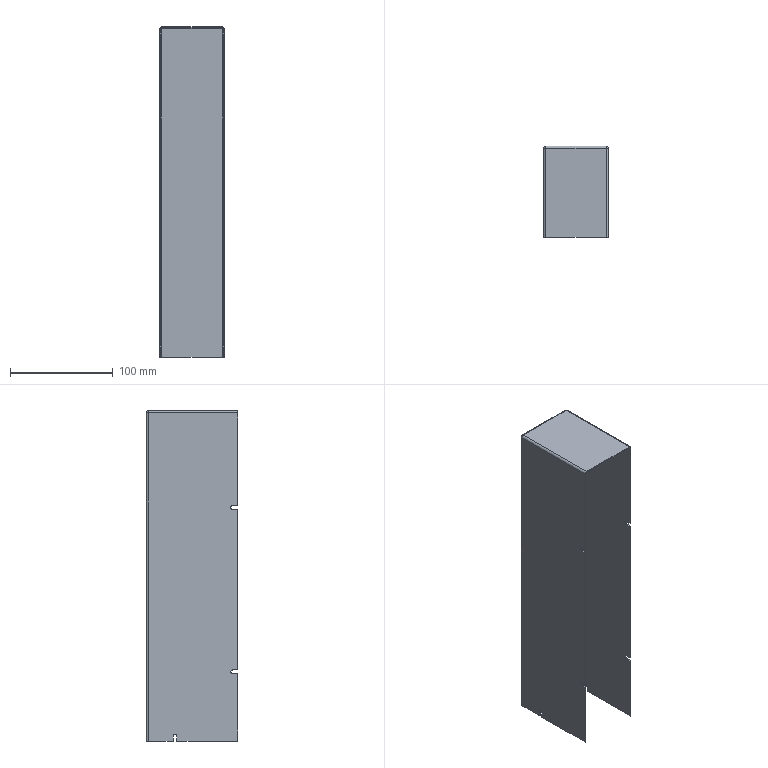Part | NX | features BREP 1 | 1 solid | 48 faces | box 63 x 89 x 321.5 mm | volume 81505 mm3 | plane 28 | cylinder 16 | sphere 4 | commonest cylinder face diameters 3.5 x6 2 x5 4 x5
STEP:
#1=CARTESIAN_POINT('',(30.5,14.75,0.));
#2=VERTEX_POINT('',#1);
#3=CARTESIAN_POINT('',(30.5,14.75,5.));
#4=VERTEX_POINT('',#3);
#5=CARTESIAN_POINT('',(30.5,14.75,321.5));
#6=DIRECTION('',(0.,0.,1.));
#7=VECTOR('',#6,1000.);
#8=LINE('',#5,#7);
#9=EDGE_CURVE('',#2,#4,#8,.T.);
#10=ORIENTED_EDGE('',*,*,#9,.T.);
#11=CARTESIAN_POINT('',(31.5,14.75,5.));
#12=VERTEX_POINT('',#11);
#13=CARTESIAN_POINT('',(-31.5,14.75,5.));
#14=DIRECTION('',(1.,0.,0.));
#15=VECTOR('',#14,1000.);
#16=LINE('',#13,#15);
#17=EDGE_CURVE('',#4,#12,#16,.T.);
#18=ORIENTED_EDGE('',*,*,#17,.T.);
#19=CARTESIAN_POINT('',(31.5,14.75,0.));
#20=VERTEX_POINT('',#19);
#21=CARTESIAN_POINT('',(31.5,14.75,5.));
#22=DIRECTION('',(0.,0.,-1.));
#23=VECTOR('',#22,1000.);
#24=LINE('',#21,#23);
#25=EDGE_CURVE('',#12,#20,#24,.T.);
#26=ORIENTED_EDGE('',*,*,#25,.T.);
#27=CARTESIAN_POINT('',(-31.5,14.75,0.));
#28=DIRECTION('',(1.,0.,0.));
#29=VECTOR('',#28,1000.);
#30=LINE('',#27,#29);
#31=EDGE_CURVE('',#2,#20,#30,.T.);
#32=ORIENTED_EDGE('',*,*,#31,.F.);
#33=EDGE_LOOP('',(#10,#18,#26,#32));
#34=FACE_BOUND('',#33,.T.);
#35=CARTESIAN_POINT('',(-31.5,14.75,5.));
#36=DIRECTION('',(0.,-1.,0.));
#37=DIRECTION('',(0.,0.,-1.));
#38=AXIS2_PLACEMENT_3D('',#35,#36,#37);
#39=PLANE('',#38);
#40=ADVANCED_FACE('',(#34),#39,.F.);
#41=CARTESIAN_POINT('',(30.5,18.25,5.));
#42=VERTEX_POINT('',#41);
#43=CARTESIAN_POINT('',(30.5,18.25,0.));
#44=VERTEX_POINT('',#43);
#45=CARTESIAN_POINT('',(30.5,18.25,321.5));
#46=DIRECTION('',(0.,0.,-1.));
#47=VECTOR('',#46,1000.);
#48=LINE('',#45,#47);
#49=EDGE_CURVE('',#42,#44,#48,.T.);
#50=ORIENTED_EDGE('',*,*,#49,.T.);
#51=CARTESIAN_POINT('',(31.5,18.25,0.));
#52=VERTEX_POINT('',#51);
#53=CARTESIAN_POINT('',(-31.5,18.25,0.));
#54=DIRECTION('',(1.,0.,0.));
#55=VECTOR('',#54,1000.);
#56=LINE('',#53,#55);
#57=EDGE_CURVE('',#44,#52,#56,.T.);
#58=ORIENTED_EDGE('',*,*,#57,.T.);
#59=CARTESIAN_POINT('',(31.5,18.25,5.));
#60=VERTEX_POINT('',#59);
#61=CARTESIAN_POINT('',(31.5,18.25,5.));
#62=DIRECTION('',(0.,0.,1.));
#63=VECTOR('',#62,1000.);
#64=LINE('',#61,#63);
#65=EDGE_CURVE('',#52,#60,#64,.T.);
#66=ORIENTED_EDGE('',*,*,#65,.T.);
#67=CARTESIAN_POINT('',(-31.5,18.25,5.));
#68=DIRECTION('',(1.,0.,0.));
#69=VECTOR('',#68,1000.);
#70=LINE('',#67,#69);
#71=EDGE_CURVE('',#42,#60,#70,.T.);
#72=ORIENTED_EDGE('',*,*,#71,.F.);
#73=EDGE_LOOP('',(#50,#58,#66,#72));
#74=FACE_BOUND('',#73,.T.);
#75=CARTESIAN_POINT('',(-31.5,18.25,5.));
#76=DIRECTION('',(0.,1.,0.));
#77=DIRECTION('',(0.,0.,1.));
#78=AXIS2_PLACEMENT_3D('',#75,#76,#77);
#79=PLANE('',#78);
#80=ADVANCED_FACE('',(#74),#79,.F.);
#81=CARTESIAN_POINT('',(30.5,16.5,5.));
#82=DIRECTION('',(-1.,0.,0.));
#83=DIRECTION('',(0.,0.,1.));
#84=AXIS2_PLACEMENT_3D('',#81,#82,#83);
#85=CIRCLE('',#84,1.75);
#86=EDGE_CURVE('',#4,#42,#85,.T.);
#87=ORIENTED_EDGE('',*,*,#86,.T.);
#88=ORIENTED_EDGE('',*,*,#71,.T.);
#89=CARTESIAN_POINT('',(31.5,16.5,5.));
#90=DIRECTION('',(1.,0.,0.));
#91=DIRECTION('',(0.,0.,-1.));
#92=AXIS2_PLACEMENT_3D('',#89,#90,#91);
#93=CIRCLE('',#92,1.75);
#94=EDGE_CURVE('',#60,#12,#93,.T.);
#95=ORIENTED_EDGE('',*,*,#94,.T.);
#96=ORIENTED_EDGE('',*,*,#17,.F.);
#97=EDGE_LOOP('',(#87,#88,#95,#96));
#98=FACE_BOUND('',#97,.T.);
#99=CARTESIAN_POINT('',(-31.5,16.5,5.));
#100=DIRECTION('',(1.,0.,0.));
#101=DIRECTION('',(0.,0.,-1.));
#102=AXIS2_PLACEMENT_3D('',#99,#100,#101);
#103=CYLINDRICAL_SURFACE('',#102,1.75);
#104=ADVANCED_FACE('',(#98),#103,.F.);
#105=CARTESIAN_POINT('',(30.5,-44.5,69.25));
#106=VERTEX_POINT('',#105);
#107=CARTESIAN_POINT('',(30.5,-39.5,69.25));
#108=VERTEX_POINT('',#107);
#109=CARTESIAN_POINT('',(30.5,-44.5,69.25));
#110=DIRECTION('',(0.,1.,0.));
#111=VECTOR('',#110,1000.);
#112=LINE('',#109,#111);
#113=EDGE_CURVE('',#106,#108,#112,.T.);
#114=ORIENTED_EDGE('',*,*,#113,.T.);
#115=CARTESIAN_POINT('',(31.5,-39.5,69.25));
#116=VERTEX_POINT('',#115);
#117=CARTESIAN_POINT('',(-31.5,-39.5,69.25));
#118=DIRECTION('',(1.,0.,0.));
#119=VECTOR('',#118,1000.);
#120=LINE('',#117,#119);
#121=EDGE_CURVE('',#108,#116,#120,.T.);
#122=ORIENTED_EDGE('',*,*,#121,.T.);
#123=CARTESIAN_POINT('',(31.5,-44.5,69.25));
#124=VERTEX_POINT('',#123);
#125=CARTESIAN_POINT('',(31.5,-39.5,69.25));
#126=DIRECTION('',(0.,-1.,0.));
#127=VECTOR('',#126,1000.);
#128=LINE('',#125,#127);
#129=EDGE_CURVE('',#116,#124,#128,.T.);
#130=ORIENTED_EDGE('',*,*,#129,.T.);
#131=CARTESIAN_POINT('',(-31.5,-44.5,69.25));
#132=DIRECTION('',(1.,0.,0.));
#133=VECTOR('',#132,1000.);
#134=LINE('',#131,#133);
#135=EDGE_CURVE('',#106,#124,#134,.T.);
#136=ORIENTED_EDGE('',*,*,#135,.F.);
#137=EDGE_LOOP('',(#114,#122,#130,#136));
#138=FACE_BOUND('',#137,.T.);
#139=CARTESIAN_POINT('',(-31.5,-39.5,69.25));
#140=DIRECTION('',(0.,0.,1.));
#141=DIRECTION('',(0.,-1.,0.));
#142=AXIS2_PLACEMENT_3D('',#139,#140,#141);
#143=PLANE('',#142);
#144=ADVANCED_FACE('',(#138),#143,.F.);
#145=CARTESIAN_POINT('',(30.5,-39.5,65.75));
#146=VERTEX_POINT('',#145);
#147=CARTESIAN_POINT('',(30.5,-44.5,65.75));
#148=VERTEX_POINT('',#147);
#149=CARTESIAN_POINT('',(30.5,-44.5,65.75));
#150=DIRECTION('',(0.,-1.,0.));
#151=VECTOR('',#150,1000.);
#152=LINE('',#149,#151);
#153=EDGE_CURVE('',#146,#148,#152,.T.);
#154=ORIENTED_EDGE('',*,*,#153,.T.);
#155=CARTESIAN_POINT('',(31.5,-44.5,65.75));
#156=VERTEX_POINT('',#155);
#157=CARTESIAN_POINT('',(-31.5,-44.5,65.75));
#158=DIRECTION('',(1.,0.,0.));
#159=VECTOR('',#158,1000.);
#160=LINE('',#157,#159);
#161=EDGE_CURVE('',#148,#156,#160,.T.);
#162=ORIENTED_EDGE('',*,*,#161,.T.);
#163=CARTESIAN_POINT('',(31.5,-39.5,65.75));
#164=VERTEX_POINT('',#163);
#165=CARTESIAN_POINT('',(31.5,-39.5,65.75));
#166=DIRECTION('',(0.,1.,0.));
#167=VECTOR('',#166,1000.);
#168=LINE('',#165,#167);
#169=EDGE_CURVE('',#156,#164,#168,.T.);
#170=ORIENTED_EDGE('',*,*,#169,.T.);
#171=CARTESIAN_POINT('',(-31.5,-39.5,65.75));
#172=DIRECTION('',(1.,0.,0.));
#173=VECTOR('',#172,1000.);
#174=LINE('',#171,#173);
#175=EDGE_CURVE('',#146,#164,#174,.T.);
#176=ORIENTED_EDGE('',*,*,#175,.F.);
#177=EDGE_LOOP('',(#154,#162,#170,#176));
#178=FACE_BOUND('',#177,.T.);
#179=CARTESIAN_POINT('',(-31.5,-39.5,65.75));
#180=DIRECTION('',(0.,0.,-1.));
#181=DIRECTION('',(0.,1.,0.));
#182=AXIS2_PLACEMENT_3D('',#179,#180,#181);
#183=PLANE('',#182);
#184=ADVANCED_FACE('',(#178),#183,.F.);
#185=CARTESIAN_POINT('',(30.5,-39.5,67.5));
#186=DIRECTION('',(-1.,0.,0.));
#187=DIRECTION('',(0.,0.,1.));
#188=AXIS2_PLACEMENT_3D('',#185,#186,#187);
#189=CIRCLE('',#188,1.75);
#190=EDGE_CURVE('',#108,#146,#189,.T.);
#191=ORIENTED_EDGE('',*,*,#190,.T.);
#192=ORIENTED_EDGE('',*,*,#175,.T.);
#193=CARTESIAN_POINT('',(31.5,-39.5,67.5));
#194=DIRECTION('',(1.,0.,0.));
#195=DIRECTION('',(0.,0.,-1.));
#196=AXIS2_PLACEMENT_3D('',#193,#194,#195);
#197=CIRCLE('',#196,1.75);
#198=EDGE_CURVE('',#164,#116,#197,.T.);
#199=ORIENTED_EDGE('',*,*,#198,.T.);
#200=ORIENTED_EDGE('',*,*,#121,.F.);
#201=EDGE_LOOP('',(#191,#192,#199,#200));
#202=FACE_BOUND('',#201,.T.);
#203=CARTESIAN_POINT('',(-31.5,-39.5,67.5));
#204=DIRECTION('',(1.,0.,0.));
#205=DIRECTION('',(0.,0.,-1.));
#206=AXIS2_PLACEMENT_3D('',#203,#204,#205);
#207=CYLINDRICAL_SURFACE('',#206,1.75);
#208=ADVANCED_FACE('',(#202),#207,.F.);
#209=CARTESIAN_POINT('',(-30.5,18.25,5.));
#210=VERTEX_POINT('',#209);
#211=CARTESIAN_POINT('',(-30.5,14.75,5.));
#212=VERTEX_POINT('',#211);
#213=CARTESIAN_POINT('',(-30.5,16.5,5.));
#214=DIRECTION('',(1.,0.,0.));
#215=DIRECTION('',(0.,0.,-1.));
#216=AXIS2_PLACEMENT_3D('',#213,#214,#215);
#217=CIRCLE('',#216,1.75);
#218=EDGE_CURVE('',#210,#212,#217,.T.);
#219=ORIENTED_EDGE('',*,*,#218,.T.);
#220=CARTESIAN_POINT('',(-31.5,14.75,5.));
#221=VERTEX_POINT('',#220);
#222=CARTESIAN_POINT('',(-31.5,14.75,5.));
#223=DIRECTION('',(1.,0.,0.));
#224=VECTOR('',#223,1000.);
#225=LINE('',#222,#224);
#226=EDGE_CURVE('',#221,#212,#225,.T.);
#227=ORIENTED_EDGE('',*,*,#226,.F.);
#228=CARTESIAN_POINT('',(-31.5,18.25,5.));
#229=VERTEX_POINT('',#228);
#230=CARTESIAN_POINT('',(-31.5,16.5,5.));
#231=DIRECTION('',(1.,0.,0.));
#232=DIRECTION('',(0.,0.,-1.));
#233=AXIS2_PLACEMENT_3D('',#230,#231,#232);
#234=CIRCLE('',#233,1.75);
#235=EDGE_CURVE('',#229,#221,#234,.T.);
#236=ORIENTED_EDGE('',*,*,#235,.F.);
#237=CARTESIAN_POINT('',(-31.5,18.25,5.));
#238=DIRECTION('',(1.,0.,0.));
#239=VECTOR('',#238,1000.);
#240=LINE('',#237,#239);
#241=EDGE_CURVE('',#229,#210,#240,.T.);
#242=ORIENTED_EDGE('',*,*,#241,.T.);
#243=EDGE_LOOP('',(#219,#227,#236,#242));
#244=FACE_BOUND('',#243,.T.);
#245=CARTESIAN_POINT('',(-31.5,16.5,5.));
#246=DIRECTION('',(1.,0.,0.));
#247=DIRECTION('',(0.,0.,-1.));
#248=AXIS2_PLACEMENT_3D('',#245,#246,#247);
#249=CYLINDRICAL_SURFACE('',#248,1.75);
#250=ADVANCED_FACE('',(#244),#249,.F.);
#251=CARTESIAN_POINT('',(-30.5,18.25,0.));
#252=VERTEX_POINT('',#251);
#253=CARTESIAN_POINT('',(-30.5,18.25,321.5));
#254=DIRECTION('',(0.,0.,1.));
#255=VECTOR('',#254,1000.);
#256=LINE('',#253,#255);
#257=EDGE_CURVE('',#252,#210,#256,.T.);
#258=ORIENTED_EDGE('',*,*,#257,.T.);
#259=ORIENTED_EDGE('',*,*,#241,.F.);
#260=CARTESIAN_POINT('',(-31.5,18.25,0.));
#261=VERTEX_POINT('',#260);
#262=CARTESIAN_POINT('',(-31.5,18.25,5.));
#263=DIRECTION('',(0.,0.,1.));
#264=VECTOR('',#263,1000.);
#265=LINE('',#262,#264);
#266=EDGE_CURVE('',#261,#229,#265,.T.);
#267=ORIENTED_EDGE('',*,*,#266,.F.);
#268=CARTESIAN_POINT('',(-31.5,18.25,0.));
#269=DIRECTION('',(1.,0.,0.));
#270=VECTOR('',#269,1000.);
#271=LINE('',#268,#270);
#272=EDGE_CURVE('',#261,#252,#271,.T.);
#273=ORIENTED_EDGE('',*,*,#272,.T.);
#274=EDGE_LOOP('',(#258,#259,#267,#273));
#275=FACE_BOUND('',#274,.T.);
#276=CARTESIAN_POINT('',(-31.5,18.25,5.));
#277=DIRECTION('',(0.,1.,0.));
#278=DIRECTION('',(0.,0.,1.));
#279=AXIS2_PLACEMENT_3D('',#276,#277,#278);
#280=PLANE('',#279);
#281=ADVANCED_FACE('',(#275),#280,.F.);
#282=CARTESIAN_POINT('',(-30.5,14.75,0.));
#283=VERTEX_POINT('',#282);
#284=CARTESIAN_POINT('',(-30.5,14.75,321.5));
#285=DIRECTION('',(0.,0.,-1.));
#286=VECTOR('',#285,1000.);
#287=LINE('',#284,#286);
#288=EDGE_CURVE('',#212,#283,#287,.T.);
#289=ORIENTED_EDGE('',*,*,#288,.T.);
#290=CARTESIAN_POINT('',(-31.5,14.75,0.));
#291=VERTEX_POINT('',#290);
#292=CARTESIAN_POINT('',(-31.5,14.75,0.));
#293=DIRECTION('',(1.,0.,0.));
#294=VECTOR('',#293,1000.);
#295=LINE('',#292,#294);
#296=EDGE_CURVE('',#291,#283,#295,.T.);
#297=ORIENTED_EDGE('',*,*,#296,.F.);
#298=CARTESIAN_POINT('',(-31.5,14.75,5.));
#299=DIRECTION('',(0.,0.,-1.));
#300=VECTOR('',#299,1000.);
#301=LINE('',#298,#300);
#302=EDGE_CURVE('',#221,#291,#301,.T.);
#303=ORIENTED_EDGE('',*,*,#302,.F.);
#304=ORIENTED_EDGE('',*,*,#226,.T.);
#305=EDGE_LOOP('',(#289,#297,#303,#304));
#306=FACE_BOUND('',#305,.T.);
#307=CARTESIAN_POINT('',(-31.5,14.75,5.));
#308=DIRECTION('',(0.,-1.,0.));
#309=DIRECTION('',(0.,0.,-1.));
#310=AXIS2_PLACEMENT_3D('',#307,#308,#309);
#311=PLANE('',#310);
#312=ADVANCED_FACE('',(#306),#311,.F.);
#313=CARTESIAN_POINT('',(-30.5,-39.5,65.75));
#314=VERTEX_POINT('',#313);
#315=CARTESIAN_POINT('',(-30.5,-39.5,69.25));
#316=VERTEX_POINT('',#315);
#317=CARTESIAN_POINT('',(-30.5,-39.5,67.5));
#318=DIRECTION('',(1.,0.,0.));
#319=DIRECTION('',(0.,0.,-1.));
#320=AXIS2_PLACEMENT_3D('',#317,#318,#319);
#321=CIRCLE('',#320,1.75);
#322=EDGE_CURVE('',#314,#316,#321,.T.);
#323=ORIENTED_EDGE('',*,*,#322,.T.);
#324=CARTESIAN_POINT('',(-31.5,-39.5,69.25));
#325=VERTEX_POINT('',#324);
#326=CARTESIAN_POINT('',(-31.5,-39.5,69.25));
#327=DIRECTION('',(1.,0.,0.));
#328=VECTOR('',#327,1000.);
#329=LINE('',#326,#328);
#330=EDGE_CURVE('',#325,#316,#329,.T.);
#331=ORIENTED_EDGE('',*,*,#330,.F.);
#332=CARTESIAN_POINT('',(-31.5,-39.5,65.75));
#333=VERTEX_POINT('',#332);
#334=CARTESIAN_POINT('',(-31.5,-39.5,67.5));
#335=DIRECTION('',(1.,0.,0.));
#336=DIRECTION('',(0.,0.,-1.));
#337=AXIS2_PLACEMENT_3D('',#334,#335,#336);
#338=CIRCLE('',#337,1.75);
#339=EDGE_CURVE('',#333,#325,#338,.T.);
#340=ORIENTED_EDGE('',*,*,#339,.F.);
#341=CARTESIAN_POINT('',(-31.5,-39.5,65.75));
#342=DIRECTION('',(1.,0.,0.));
#343=VECTOR('',#342,1000.);
#344=LINE('',#341,#343);
#345=EDGE_CURVE('',#333,#314,#344,.T.);
#346=ORIENTED_EDGE('',*,*,#345,.T.);
#347=EDGE_LOOP('',(#323,#331,#340,#346));
#348=FACE_BOUND('',#347,.T.);
#349=CARTESIAN_POINT('',(-31.5,-39.5,67.5));
#350=DIRECTION('',(1.,0.,0.));
#351=DIRECTION('',(0.,0.,-1.));
#352=AXIS2_PLACEMENT_3D('',#349,#350,#351);
#353=CYLINDRICAL_SURFACE('',#352,1.75);
#354=ADVANCED_FACE('',(#348),#353,.F.);
#355=CARTESIAN_POINT('',(-30.5,-44.5,65.75));
#356=VERTEX_POINT('',#355);
#357=CARTESIAN_POINT('',(-30.5,-44.5,65.75));
#358=DIRECTION('',(0.,1.,0.));
#359=VECTOR('',#358,1000.);
#360=LINE('',#357,#359);
#361=EDGE_CURVE('',#356,#314,#360,.T.);
#362=ORIENTED_EDGE('',*,*,#361,.T.);
#363=ORIENTED_EDGE('',*,*,#345,.F.);
#364=CARTESIAN_POINT('',(-31.5,-44.5,65.75));
#365=VERTEX_POINT('',#364);
#366=CARTESIAN_POINT('',(-31.5,-39.5,65.75));
#367=DIRECTION('',(0.,1.,0.));
#368=VECTOR('',#367,1000.);
#369=LINE('',#366,#368);
#370=EDGE_CURVE('',#365,#333,#369,.T.);
#371=ORIENTED_EDGE('',*,*,#370,.F.);
#372=CARTESIAN_POINT('',(-31.5,-44.5,65.75));
#373=DIRECTION('',(1.,0.,0.));
#374=VECTOR('',#373,1000.);
#375=LINE('',#372,#374);
#376=EDGE_CURVE('',#365,#356,#375,.T.);
#377=ORIENTED_EDGE('',*,*,#376,.T.);
#378=EDGE_LOOP('',(#362,#363,#371,#377));
#379=FACE_BOUND('',#378,.T.);
#380=CARTESIAN_POINT('',(-31.5,-39.5,65.75));
#381=DIRECTION('',(0.,0.,-1.));
#382=DIRECTION('',(0.,1.,0.));
#383=AXIS2_PLACEMENT_3D('',#380,#381,#382);
#384=PLANE('',#383);
#385=ADVANCED_FACE('',(#379),#384,.F.);
#386=CARTESIAN_POINT('',(-30.5,-44.5,69.25));
#387=VERTEX_POINT('',#386);
#388=CARTESIAN_POINT('',(-30.5,-44.5,69.25));
#389=DIRECTION('',(0.,-1.,0.));
#390=VECTOR('',#389,1000.);
#391=LINE('',#388,#390);
#392=EDGE_CURVE('',#316,#387,#391,.T.);
#393=ORIENTED_EDGE('',*,*,#392,.T.);
#394=CARTESIAN_POINT('',(-31.5,-44.5,69.25));
#395=VERTEX_POINT('',#394);
#396=CARTESIAN_POINT('',(-31.5,-44.5,69.25));
#397=DIRECTION('',(1.,0.,0.));
#398=VECTOR('',#397,1000.);
#399=LINE('',#396,#398);
#400=EDGE_CURVE('',#395,#387,#399,.T.);
#401=ORIENTED_EDGE('',*,*,#400,.F.);
#402=CARTESIAN_POINT('',(-31.5,-39.5,69.25));
#403=DIRECTION('',(0.,-1.,0.));
#404=VECTOR('',#403,1000.);
#405=LINE('',#402,#404);
#406=EDGE_CURVE('',#325,#395,#405,.T.);
#407=ORIENTED_EDGE('',*,*,#406,.F.);
#408=ORIENTED_EDGE('',*,*,#330,.T.);
#409=EDGE_LOOP('',(#393,#401,#407,#408));
#410=FACE_BOUND('',#409,.T.);
#411=CARTESIAN_POINT('',(-31.5,-39.5,69.25));
#412=DIRECTION('',(0.,0.,1.));
#413=DIRECTION('',(0.,-1.,0.));
#414=AXIS2_PLACEMENT_3D('',#411,#412,#413);
#415=PLANE('',#414);
#416=ADVANCED_FACE('',(#410),#415,.F.);
#417=CARTESIAN_POINT('',(30.5,-39.5,225.75));
#418=VERTEX_POINT('',#417);
#419=CARTESIAN_POINT('',(30.5,-44.5,225.75));
#420=VERTEX_POINT('',#419);
#421=CARTESIAN_POINT('',(30.5,-44.5,225.75));
#422=DIRECTION('',(0.,-1.,0.));
#423=VECTOR('',#422,1000.);
#424=LINE('',#421,#423);
#425=EDGE_CURVE('',#418,#420,#424,.T.);
#426=ORIENTED_EDGE('',*,*,#425,.T.);
#427=CARTESIAN_POINT('',(31.5,-44.5,225.75));
#428=VERTEX_POINT('',#427);
#429=CARTESIAN_POINT('',(-31.5,-44.5,225.75));
#430=DIRECTION('',(1.,0.,0.));
#431=VECTOR('',#430,1000.);
#432=LINE('',#429,#431);
#433=EDGE_CURVE('',#420,#428,#432,.T.);
#434=ORIENTED_EDGE('',*,*,#433,.T.);
#435=CARTESIAN_POINT('',(31.5,-39.5,225.75));
#436=VERTEX_POINT('',#435);
#437=CARTESIAN_POINT('',(31.5,-44.5,225.75));
#438=DIRECTION('',(0.,1.,0.));
#439=VECTOR('',#438,1000.);
#440=LINE('',#437,#439);
#441=EDGE_CURVE('',#428,#436,#440,.T.);
#442=ORIENTED_EDGE('',*,*,#441,.T.);
#443=CARTESIAN_POINT('',(-31.5,-39.5,225.75));
#444=DIRECTION('',(1.,0.,0.));
#445=VECTOR('',#444,1000.);
#446=LINE('',#443,#445);
#447=EDGE_CURVE('',#418,#436,#446,.T.);
#448=ORIENTED_EDGE('',*,*,#447,.F.);
#449=EDGE_LOOP('',(#426,#434,#442,#448));
#450=FACE_BOUND('',#449,.T.);
#451=CARTESIAN_POINT('',(-31.5,-44.5,225.75));
#452=DIRECTION('',(0.,0.,-1.));
#453=DIRECTION('',(0.,1.,0.));
#454=AXIS2_PLACEMENT_3D('',#451,#452,#453);
#455=PLANE('',#454);
#456=ADVANCED_FACE('',(#450),#455,.F.);
#457=CARTESIAN_POINT('',(30.5,-39.5,229.25));
#458=VERTEX_POINT('',#457);
#459=CARTESIAN_POINT('',(30.5,-39.5,227.5));
#460=DIRECTION('',(-1.,0.,0.));
#461=DIRECTION('',(0.,0.,1.));
#462=AXIS2_PLACEMENT_3D('',#459,#460,#461);
#463=CIRCLE('',#462,1.75);
#464=EDGE_CURVE('',#458,#418,#463,.T.);
#465=ORIENTED_EDGE('',*,*,#464,.T.);
#466=ORIENTED_EDGE('',*,*,#447,.T.);
#467=CARTESIAN_POINT('',(31.5,-39.5,229.25));
#468=VERTEX_POINT('',#467);
#469=CARTESIAN_POINT('',(31.5,-39.5,227.5));
#470=DIRECTION('',(1.,0.,0.));
#471=DIRECTION('',(0.,0.,-1.));
#472=AXIS2_PLACEMENT_3D('',#469,#470,#471);
#473=CIRCLE('',#472,1.75);
#474=EDGE_CURVE('',#436,#468,#473,.T.);
#475=ORIENTED_EDGE('',*,*,#474,.T.);
#476=CARTESIAN_POINT('',(-31.5,-39.5,229.25));
#477=DIRECTION('',(1.,0.,0.));
#478=VECTOR('',#477,1000.);
#479=LINE('',#476,#478);
#480=EDGE_CURVE('',#458,#468,#479,.T.);
#481=ORIENTED_EDGE('',*,*,#480,.F.);
#482=EDGE_LOOP('',(#465,#466,#475,#481));
#483=FACE_BOUND('',#482,.T.);
#484=CARTESIAN_POINT('',(-31.5,-39.5,227.5));
#485=DIRECTION('',(1.,0.,0.));
#486=DIRECTION('',(0.,0.,-1.));
#487=AXIS2_PLACEMENT_3D('',#484,#485,#486);
#488=CYLINDRICAL_SURFACE('',#487,1.75);
#489=ADVANCED_FACE('',(#483),#488,.F.);
#490=CARTESIAN_POINT('',(30.5,-44.5,229.25));
#491=VERTEX_POINT('',#490);
#492=CARTESIAN_POINT('',(30.5,-44.5,229.25));
#493=DIRECTION('',(0.,1.,0.));
#494=VECTOR('',#493,1000.);
#495=LINE('',#492,#494);
#496=EDGE_CURVE('',#491,#458,#495,.T.);
#497=ORIENTED_EDGE('',*,*,#496,.T.);
#498=ORIENTED_EDGE('',*,*,#480,.T.);
#499=CARTESIAN_POINT('',(31.5,-44.5,229.25));
#500=VERTEX_POINT('',#499);
#501=CARTESIAN_POINT('',(31.5,-44.5,229.25));
#502=DIRECTION('',(0.,-1.,0.));
#503=VECTOR('',#502,1000.);
#504=LINE('',#501,#503);
#505=EDGE_CURVE('',#468,#500,#504,.T.);
#506=ORIENTED_EDGE('',*,*,#505,.T.);
#507=CARTESIAN_POINT('',(-31.5,-44.5,229.25));
#508=DIRECTION('',(1.,0.,0.));
#509=VECTOR('',#508,1000.);
#510=LINE('',#507,#509);
#511=EDGE_CURVE('',#491,#500,#510,.T.);
#512=ORIENTED_EDGE('',*,*,#511,.F.);
#513=EDGE_LOOP('',(#497,#498,#506,#512));
#514=FACE_BOUND('',#513,.T.);
#515=CARTESIAN_POINT('',(-31.5,-44.5,229.25));
#516=DIRECTION('',(0.,0.,1.));
#517=DIRECTION('',(0.,-1.,0.));
#518=AXIS2_PLACEMENT_3D('',#515,#516,#517);
#519=PLANE('',#518);
#520=ADVANCED_FACE('',(#514),#519,.F.);
#521=CARTESIAN_POINT('',(-30.5,-39.5,229.25));
#522=VERTEX_POINT('',#521);
#523=CARTESIAN_POINT('',(-30.5,-44.5,229.25));
#524=VERTEX_POINT('',#523);
#525=CARTESIAN_POINT('',(-30.5,-44.5,229.25));
#526=DIRECTION('',(0.,-1.,0.));
#527=VECTOR('',#526,1000.);
#528=LINE('',#525,#527);
#529=EDGE_CURVE('',#522,#524,#528,.T.);
#530=ORIENTED_EDGE('',*,*,#529,.T.);
#531=CARTESIAN_POINT('',(-31.5,-44.5,229.25));
#532=VERTEX_POINT('',#531);
#533=CARTESIAN_POINT('',(-31.5,-44.5,229.25));
#534=DIRECTION('',(1.,0.,0.));
#535=VECTOR('',#534,1000.);
#536=LINE('',#533,#535);
#537=EDGE_CURVE('',#532,#524,#536,.T.);
#538=ORIENTED_EDGE('',*,*,#537,.F.);
#539=CARTESIAN_POINT('',(-31.5,-39.5,229.25));
#540=VERTEX_POINT('',#539);
#541=CARTESIAN_POINT('',(-31.5,-44.5,229.25));
#542=DIRECTION('',(0.,-1.,0.));
#543=VECTOR('',#542,1000.);
#544=LINE('',#541,#543);
#545=EDGE_CURVE('',#540,#532,#544,.T.);
#546=ORIENTED_EDGE('',*,*,#545,.F.);
#547=CARTESIAN_POINT('',(-31.5,-39.5,229.25));
#548=DIRECTION('',(1.,0.,0.));
#549=VECTOR('',#548,1000.);
#550=LINE('',#547,#549);
#551=EDGE_CURVE('',#540,#522,#550,.T.);
#552=ORIENTED_EDGE('',*,*,#551,.T.);
#553=EDGE_LOOP('',(#530,#538,#546,#552));
#554=FACE_BOUND('',#553,.T.);
#555=CARTESIAN_POINT('',(-31.5,-44.5,229.25));
#556=DIRECTION('',(0.,0.,1.));
#557=DIRECTION('',(0.,-1.,0.));
#558=AXIS2_PLACEMENT_3D('',#555,#556,#557);
#559=PLANE('',#558);
#560=ADVANCED_FACE('',(#554),#559,.F.);
#561=CARTESIAN_POINT('',(-30.5,-39.5,225.75));
#562=VERTEX_POINT('',#561);
#563=CARTESIAN_POINT('',(-30.5,-39.5,227.5));
#564=DIRECTION('',(1.,0.,0.));
#565=DIRECTION('',(0.,0.,-1.));
#566=AXIS2_PLACEMENT_3D('',#563,#564,#565);
#567=CIRCLE('',#566,1.75);
#568=EDGE_CURVE('',#562,#522,#567,.T.);
#569=ORIENTED_EDGE('',*,*,#568,.T.);
#570=ORIENTED_EDGE('',*,*,#551,.F.);
#571=CARTESIAN_POINT('',(-31.5,-39.5,225.75));
#572=VERTEX_POINT('',#571);
#573=CARTESIAN_POINT('',(-31.5,-39.5,227.5));
#574=DIRECTION('',(1.,0.,0.));
#575=DIRECTION('',(0.,0.,-1.));
#576=AXIS2_PLACEMENT_3D('',#573,#574,#575);
#577=CIRCLE('',#576,1.75);
#578=EDGE_CURVE('',#572,#540,#577,.T.);
#579=ORIENTED_EDGE('',*,*,#578,.F.);
#580=CARTESIAN_POINT('',(-31.5,-39.5,225.75));
#581=DIRECTION('',(1.,0.,0.));
#582=VECTOR('',#581,1000.);
#583=LINE('',#580,#582);
#584=EDGE_CURVE('',#572,#562,#583,.T.);
#585=ORIENTED_EDGE('',*,*,#584,.T.);
#586=EDGE_LOOP('',(#569,#570,#579,#585));
#587=FACE_BOUND('',#586,.T.);
#588=CARTESIAN_POINT('',(-31.5,-39.5,227.5));
#589=DIRECTION('',(1.,0.,0.));
#590=DIRECTION('',(0.,0.,-1.));
#591=AXIS2_PLACEMENT_3D('',#588,#589,#590);
#592=CYLINDRICAL_SURFACE('',#591,1.75);
#593=ADVANCED_FACE('',(#587),#592,.F.);
#594=CARTESIAN_POINT('',(-30.5,-44.5,225.75));
#595=VERTEX_POINT('',#594);
#596=CARTESIAN_POINT('',(-30.5,-44.5,225.75));
#597=DIRECTION('',(0.,1.,0.));
#598=VECTOR('',#597,1000.);
#599=LINE('',#596,#598);
#600=EDGE_CURVE('',#595,#562,#599,.T.);
#601=ORIENTED_EDGE('',*,*,#600,.T.);
#602=ORIENTED_EDGE('',*,*,#584,.F.);
#603=CARTESIAN_POINT('',(-31.5,-44.5,225.75));
#604=VERTEX_POINT('',#603);
#605=CARTESIAN_POINT('',(-31.5,-44.5,225.75));
#606=DIRECTION('',(0.,1.,0.));
#607=VECTOR('',#606,1000.);
#608=LINE('',#605,#607);
#609=EDGE_CURVE('',#604,#572,#608,.T.);
#610=ORIENTED_EDGE('',*,*,#609,.F.);
#611=CARTESIAN_POINT('',(-31.5,-44.5,225.75));
#612=DIRECTION('',(1.,0.,0.));
#613=VECTOR('',#612,1000.);
#614=LINE('',#611,#613);
#615=EDGE_CURVE('',#604,#595,#614,.T.);
#616=ORIENTED_EDGE('',*,*,#615,.T.);
#617=EDGE_LOOP('',(#601,#602,#610,#616));
#618=FACE_BOUND('',#617,.T.);
#619=CARTESIAN_POINT('',(-31.5,-44.5,225.75));
#620=DIRECTION('',(0.,0.,-1.));
#621=DIRECTION('',(0.,1.,0.));
#622=AXIS2_PLACEMENT_3D('',#619,#620,#621);
#623=PLANE('',#622);
#624=ADVANCED_FACE('',(#618),#623,.F.);
#625=CARTESIAN_POINT('',(29.5,42.5,320.5));
#626=VERTEX_POINT('',#625);
#627=CARTESIAN_POINT('',(29.5,43.5,319.5));
#628=VERTEX_POINT('',#627);
#629=CARTESIAN_POINT('',(29.5,42.5,319.5));
#630=DIRECTION('',(-1.,0.,0.));
#631=DIRECTION('',(0.,0.,1.));
#632=AXIS2_PLACEMENT_3D('',#629,#630,#631);
#633=CIRCLE('',#632,1.);
#634=EDGE_CURVE('',#626,#628,#633,.T.);
#635=ORIENTED_EDGE('',*,*,#634,.F.);
#636=CARTESIAN_POINT('',(-29.5,42.5,320.5));
#637=VERTEX_POINT('',#636);
#638=CARTESIAN_POINT('',(0.,42.5,320.5));
#639=DIRECTION('',(-1.,0.,0.));
#640=VECTOR('',#639,1000.);
#641=LINE('',#638,#640);
#642=EDGE_CURVE('',#626,#637,#641,.T.);
#643=ORIENTED_EDGE('',*,*,#642,.T.);
#644=CARTESIAN_POINT('',(-29.5,43.5,319.5));
#645=VERTEX_POINT('',#644);
#646=CARTESIAN_POINT('',(-29.5,42.5,319.5));
#647=DIRECTION('',(1.,0.,0.));
#648=DIRECTION('',(0.,0.,1.));
#649=AXIS2_PLACEMENT_3D('',#646,#647,#648);
#650=CIRCLE('',#649,1.);
#651=EDGE_CURVE('',#645,#637,#650,.T.);
#652=ORIENTED_EDGE('',*,*,#651,.F.);
#653=CARTESIAN_POINT('',(-31.5,43.5,319.5));
#654=DIRECTION('',(1.,0.,0.));
#655=VECTOR('',#654,1000.);
#656=LINE('',#653,#655);
#657=EDGE_CURVE('',#645,#628,#656,.T.);
#658=ORIENTED_EDGE('',*,*,#657,.T.);
#659=EDGE_LOOP('',(#635,#643,#652,#658));
#660=FACE_BOUND('',#659,.T.);
#661=CARTESIAN_POINT('',(0.,42.5,319.5));
#662=DIRECTION('',(-1.,0.,0.));
#663=DIRECTION('',(0.,0.,1.));
#664=AXIS2_PLACEMENT_3D('',#661,#662,#663);
#665=CYLINDRICAL_SURFACE('',#664,1.);
#666=ADVANCED_FACE('',(#660),#665,.F.);
#667=CARTESIAN_POINT('',(-30.5,42.5,319.5));
#668=VERTEX_POINT('',#667);
#669=CARTESIAN_POINT('',(-29.5,42.5,319.5));
#670=DIRECTION('',(0.,0.,1.));
#671=DIRECTION('',(1.,0.,0.));
#672=AXIS2_PLACEMENT_3D('',#669,#670,#671);
#673=CIRCLE('',#672,1.);
#674=EDGE_CURVE('',#645,#668,#673,.T.);
#675=ORIENTED_EDGE('',*,*,#674,.F.);
#676=ORIENTED_EDGE('',*,*,#651,.T.);
#677=CARTESIAN_POINT('',(-29.5,42.5,319.5));
#678=DIRECTION('',(0.,1.,0.));
#679=DIRECTION('',(-1.,0.,0.));
#680=AXIS2_PLACEMENT_3D('',#677,#678,#679);
#681=CIRCLE('',#680,1.);
#682=EDGE_CURVE('',#668,#637,#681,.T.);
#683=ORIENTED_EDGE('',*,*,#682,.F.);
#684=EDGE_LOOP('',(#675,#676,#683));
#685=FACE_BOUND('',#684,.T.);
#686=CARTESIAN_POINT('',(-29.5,42.5,319.5));
#687=DIRECTION('',(0.,1.,0.));
#688=DIRECTION('',(1.,0.,0.));
#689=AXIS2_PLACEMENT_3D('',#686,#687,#688);
#690=SPHERICAL_SURFACE('',#689,1.);
#691=ADVANCED_FACE('',(#685),#690,.F.);
#692=CARTESIAN_POINT('',(30.5,42.5,319.5));
#693=VERTEX_POINT('',#692);
#694=CARTESIAN_POINT('',(29.5,42.5,319.5));
#695=DIRECTION('',(0.,1.,0.));
#696=DIRECTION('',(0.,0.,-1.));
#697=AXIS2_PLACEMENT_3D('',#694,#695,#696);
#698=CIRCLE('',#697,1.);
#699=EDGE_CURVE('',#626,#693,#698,.T.);
#700=ORIENTED_EDGE('',*,*,#699,.F.);
#701=ORIENTED_EDGE('',*,*,#634,.T.);
#702=CARTESIAN_POINT('',(29.5,42.5,319.5));
#703=DIRECTION('',(0.,0.,1.));
#704=DIRECTION('',(1.,0.,0.));
#705=AXIS2_PLACEMENT_3D('',#702,#703,#704);
#706=CIRCLE('',#705,1.);
#707=EDGE_CURVE('',#693,#628,#706,.T.);
#708=ORIENTED_EDGE('',*,*,#707,.F.);
#709=EDGE_LOOP('',(#700,#701,#708));
#710=FACE_BOUND('',#709,.T.);
#711=CARTESIAN_POINT('',(29.5,42.5,319.5));
#712=DIRECTION('',(0.,1.,0.));
#713=DIRECTION('',(1.,0.,0.));
#714=AXIS2_PLACEMENT_3D('',#711,#712,#713);
#715=SPHERICAL_SURFACE('',#714,1.);
#716=ADVANCED_FACE('',(#710),#715,.F.);
#717=CARTESIAN_POINT('',(-30.5,42.5,0.));
#718=VERTEX_POINT('',#717);
#719=CARTESIAN_POINT('',(-29.5,43.5,0.));
#720=VERTEX_POINT('',#719);
#721=CARTESIAN_POINT('',(-29.5,42.5,0.));
#722=DIRECTION('',(0.,0.,-1.));
#723=DIRECTION('',(-1.,0.,0.));
#724=AXIS2_PLACEMENT_3D('',#721,#722,#723);
#725=CIRCLE('',#724,1.);
#726=EDGE_CURVE('',#718,#720,#725,.T.);
#727=ORIENTED_EDGE('',*,*,#726,.T.);
#728=CARTESIAN_POINT('',(-29.5,43.5,321.5));
#729=DIRECTION('',(0.,0.,1.));
#730=VECTOR('',#729,1000.);
#731=LINE('',#728,#730);
#732=EDGE_CURVE('',#720,#645,#731,.T.);
#733=ORIENTED_EDGE('',*,*,#732,.T.);
#734=ORIENTED_EDGE('',*,*,#674,.T.);
#735=CARTESIAN_POINT('',(-30.5,42.5,321.5));
#736=DIRECTION('',(0.,0.,-1.));
#737=VECTOR('',#736,1000.);
#738=LINE('',#735,#737);
#739=EDGE_CURVE('',#668,#718,#738,.T.);
#740=ORIENTED_EDGE('',*,*,#739,.T.);
#741=EDGE_LOOP('',(#727,#733,#734,#740));
#742=FACE_BOUND('',#741,.T.);
#743=CARTESIAN_POINT('',(-29.5,42.5,321.5));
#744=DIRECTION('',(0.,0.,-1.));
#745=DIRECTION('',(-1.,0.,0.));
#746=AXIS2_PLACEMENT_3D('',#743,#744,#745);
#747=CYLINDRICAL_SURFACE('',#746,1.);
#748=ADVANCED_FACE('',(#742),#747,.F.);
#749=CARTESIAN_POINT('',(-29.5,-44.5,320.5));
#750=VERTEX_POINT('',#749);
#751=CARTESIAN_POINT('',(-30.5,-44.5,319.5));
#752=VERTEX_POINT('',#751);
#753=CARTESIAN_POINT('',(-29.5,-44.5,319.5));
#754=DIRECTION('',(0.,-1.,0.));
#755=DIRECTION('',(0.,0.,1.));
#756=AXIS2_PLACEMENT_3D('',#753,#754,#755);
#757=CIRCLE('',#756,1.);
#758=EDGE_CURVE('',#750,#752,#757,.T.);
#759=ORIENTED_EDGE('',*,*,#758,.T.);
#760=CARTESIAN_POINT('',(-30.5,-44.5,319.5));
#761=DIRECTION('',(0.,1.,0.));
#762=VECTOR('',#761,1000.);
#763=LINE('',#760,#762);
#764=EDGE_CURVE('',#752,#668,#763,.T.);
#765=ORIENTED_EDGE('',*,*,#764,.T.);
#766=ORIENTED_EDGE('',*,*,#682,.T.);
#767=CARTESIAN_POINT('',(-29.5,0.,320.5));
#768=DIRECTION('',(0.,-1.,0.));
#769=VECTOR('',#768,1000.);
#770=LINE('',#767,#769);
#771=EDGE_CURVE('',#637,#750,#770,.T.);
#772=ORIENTED_EDGE('',*,*,#771,.T.);
#773=EDGE_LOOP('',(#759,#765,#766,#772));
#774=FACE_BOUND('',#773,.T.);
#775=CARTESIAN_POINT('',(-29.5,0.,319.5));
#776=DIRECTION('',(0.,-1.,0.));
#777=DIRECTION('',(0.,0.,-1.));
#778=AXIS2_PLACEMENT_3D('',#775,#776,#777);
#779=CYLINDRICAL_SURFACE('',#778,1.);
#780=ADVANCED_FACE('',(#774),#779,.F.);
#781=CARTESIAN_POINT('',(30.5,-44.5,319.5));
#782=VERTEX_POINT('',#781);
#783=CARTESIAN_POINT('',(29.5,-44.5,320.5));
#784=VERTEX_POINT('',#783);
#785=CARTESIAN_POINT('',(29.5,-44.5,319.5));
#786=DIRECTION('',(0.,-1.,0.));
#787=DIRECTION('',(0.,0.,1.));
#788=AXIS2_PLACEMENT_3D('',#785,#786,#787);
#789=CIRCLE('',#788,1.);
#790=EDGE_CURVE('',#782,#784,#789,.T.);
#791=ORIENTED_EDGE('',*,*,#790,.T.);
#792=CARTESIAN_POINT('',(29.5,0.,320.5));
#793=DIRECTION('',(0.,1.,0.));
#794=VECTOR('',#793,1000.);
#795=LINE('',#792,#794);
#796=EDGE_CURVE('',#784,#626,#795,.T.);
#797=ORIENTED_EDGE('',*,*,#796,.T.);
#798=ORIENTED_EDGE('',*,*,#699,.T.);
#799=CARTESIAN_POINT('',(30.5,-44.5,319.5));
#800=DIRECTION('',(0.,-1.,0.));
#801=VECTOR('',#800,1000.);
#802=LINE('',#799,#801);
#803=EDGE_CURVE('',#693,#782,#802,.T.);
#804=ORIENTED_EDGE('',*,*,#803,.T.);
#805=EDGE_LOOP('',(#791,#797,#798,#804));
#806=FACE_BOUND('',#805,.T.);
#807=CARTESIAN_POINT('',(29.5,0.,319.5));
#808=DIRECTION('',(0.,1.,0.));
#809=DIRECTION('',(0.,0.,1.));
#810=AXIS2_PLACEMENT_3D('',#807,#808,#809);
#811=CYLINDRICAL_SURFACE('',#810,1.);
#812=ADVANCED_FACE('',(#806),#811,.F.);
#813=CARTESIAN_POINT('',(29.5,43.5,0.));
#814=VERTEX_POINT('',#813);
#815=CARTESIAN_POINT('',(30.5,42.5,0.));
#816=VERTEX_POINT('',#815);
#817=CARTESIAN_POINT('',(29.5,42.5,0.));
#818=DIRECTION('',(0.,0.,-1.));
#819=DIRECTION('',(-1.,0.,0.));
#820=AXIS2_PLACEMENT_3D('',#817,#818,#819);
#821=CIRCLE('',#820,1.);
#822=EDGE_CURVE('',#814,#816,#821,.T.);
#823=ORIENTED_EDGE('',*,*,#822,.T.);
#824=CARTESIAN_POINT('',(30.5,42.5,321.5));
#825=DIRECTION('',(0.,0.,1.));
#826=VECTOR('',#825,1000.);
#827=LINE('',#824,#826);
#828=EDGE_CURVE('',#816,#693,#827,.T.);
#829=ORIENTED_EDGE('',*,*,#828,.T.);
#830=ORIENTED_EDGE('',*,*,#707,.T.);
#831=CARTESIAN_POINT('',(29.5,43.5,321.5));
#832=DIRECTION('',(0.,0.,-1.));
#833=VECTOR('',#832,1000.);
#834=LINE('',#831,#833);
#835=EDGE_CURVE('',#628,#814,#834,.T.);
#836=ORIENTED_EDGE('',*,*,#835,.T.);
#837=EDGE_LOOP('',(#823,#829,#830,#836));
#838=FACE_BOUND('',#837,.T.);
#839=CARTESIAN_POINT('',(29.5,42.5,321.5));
#840=DIRECTION('',(0.,0.,-1.));
#841=DIRECTION('',(-1.,0.,0.));
#842=AXIS2_PLACEMENT_3D('',#839,#840,#841);
#843=CYLINDRICAL_SURFACE('',#842,1.);
#844=ADVANCED_FACE('',(#838),#843,.F.);
#845=CARTESIAN_POINT('',(0.,-44.5,320.5));
#846=DIRECTION('',(1.,0.,0.));
#847=VECTOR('',#846,1000.);
#848=LINE('',#845,#847);
#849=EDGE_CURVE('',#750,#784,#848,.T.);
#850=ORIENTED_EDGE('',*,*,#849,.F.);
#851=ORIENTED_EDGE('',*,*,#771,.F.);
#852=ORIENTED_EDGE('',*,*,#642,.F.);
#853=ORIENTED_EDGE('',*,*,#796,.F.);
#854=EDGE_LOOP('',(#850,#851,#852,#853));
#855=FACE_BOUND('',#854,.T.);
#856=CARTESIAN_POINT('',(0.,0.,320.5));
#857=DIRECTION('',(0.,0.,-1.));
#858=DIRECTION('',(-1.,0.,0.));
#859=AXIS2_PLACEMENT_3D('',#856,#857,#858);
#860=PLANE('',#859);
#861=ADVANCED_FACE('',(#855),#860,.T.);
#862=ORIENTED_EDGE('',*,*,#257,.F.);
#863=CARTESIAN_POINT('',(-30.5,0.,0.));
#864=DIRECTION('',(0.,-1.,0.));
#865=VECTOR('',#864,1000.);
#866=LINE('',#863,#865);
#867=EDGE_CURVE('',#718,#252,#866,.T.);
#868=ORIENTED_EDGE('',*,*,#867,.F.);
#869=ORIENTED_EDGE('',*,*,#739,.F.);
#870=ORIENTED_EDGE('',*,*,#764,.F.);
#871=CARTESIAN_POINT('',(-30.5,-44.5,321.5));
#872=DIRECTION('',(0.,0.,-1.));
#873=VECTOR('',#872,1000.);
#874=LINE('',#871,#873);
#875=EDGE_CURVE('',#752,#524,#874,.T.);
#876=ORIENTED_EDGE('',*,*,#875,.T.);
#877=ORIENTED_EDGE('',*,*,#529,.F.);
#878=ORIENTED_EDGE('',*,*,#568,.F.);
#879=ORIENTED_EDGE('',*,*,#600,.F.);
#880=CARTESIAN_POINT('',(-30.5,-44.5,321.5));
#881=DIRECTION('',(0.,0.,-1.));
#882=VECTOR('',#881,1000.);
#883=LINE('',#880,#882);
#884=EDGE_CURVE('',#595,#387,#883,.T.);
#885=ORIENTED_EDGE('',*,*,#884,.T.);
#886=ORIENTED_EDGE('',*,*,#392,.F.);
#887=ORIENTED_EDGE('',*,*,#322,.F.);
#888=ORIENTED_EDGE('',*,*,#361,.F.);
#889=CARTESIAN_POINT('',(-30.5,-44.5,0.));
#890=VERTEX_POINT('',#889);
#891=CARTESIAN_POINT('',(-30.5,-44.5,321.5));
#892=DIRECTION('',(0.,0.,-1.));
#893=VECTOR('',#892,1000.);
#894=LINE('',#891,#893);
#895=EDGE_CURVE('',#356,#890,#894,.T.);
#896=ORIENTED_EDGE('',*,*,#895,.T.);
#897=CARTESIAN_POINT('',(-30.5,0.,0.));
#898=DIRECTION('',(0.,-1.,0.));
#899=VECTOR('',#898,1000.);
#900=LINE('',#897,#899);
#901=EDGE_CURVE('',#283,#890,#900,.T.);
#902=ORIENTED_EDGE('',*,*,#901,.F.);
#903=ORIENTED_EDGE('',*,*,#288,.F.);
#904=ORIENTED_EDGE('',*,*,#218,.F.);
#905=EDGE_LOOP('',(#862,#868,#869,#870,#876,#877,#878,#879,#885,#886,#887,#888,#896,#902,#903,#904));
#906=FACE_BOUND('',#905,.T.);
#907=CARTESIAN_POINT('',(-30.5,-44.5,321.5));
#908=DIRECTION('',(1.,0.,0.));
#909=DIRECTION('',(0.,0.,-1.));
#910=AXIS2_PLACEMENT_3D('',#907,#908,#909);
#911=PLANE('',#910);
#912=ADVANCED_FACE('',(#906),#911,.T.);
#913=CARTESIAN_POINT('',(0.,43.5,0.));
#914=DIRECTION('',(-1.,0.,0.));
#915=VECTOR('',#914,1000.);
#916=LINE('',#913,#915);
#917=EDGE_CURVE('',#814,#720,#916,.T.);
#918=ORIENTED_EDGE('',*,*,#917,.F.);
#919=ORIENTED_EDGE('',*,*,#835,.F.);
#920=ORIENTED_EDGE('',*,*,#657,.F.);
#921=ORIENTED_EDGE('',*,*,#732,.F.);
#922=EDGE_LOOP('',(#918,#919,#920,#921));
#923=FACE_BOUND('',#922,.T.);
#924=CARTESIAN_POINT('',(-31.5,43.5,321.5));
#925=DIRECTION('',(0.,-1.,0.));
#926=DIRECTION('',(0.,0.,-1.));
#927=AXIS2_PLACEMENT_3D('',#924,#925,#926);
#928=PLANE('',#927);
#929=ADVANCED_FACE('',(#923),#928,.T.);
#930=ORIENTED_EDGE('',*,*,#49,.F.);
#931=ORIENTED_EDGE('',*,*,#86,.F.);
#932=ORIENTED_EDGE('',*,*,#9,.F.);
#933=CARTESIAN_POINT('',(30.5,-44.5,0.));
#934=VERTEX_POINT('',#933);
#935=CARTESIAN_POINT('',(30.5,0.,0.));
#936=DIRECTION('',(0.,1.,0.));
#937=VECTOR('',#936,1000.);
#938=LINE('',#935,#937);
#939=EDGE_CURVE('',#934,#2,#938,.T.);
#940=ORIENTED_EDGE('',*,*,#939,.F.);
#941=CARTESIAN_POINT('',(30.5,-44.5,321.5));
#942=DIRECTION('',(0.,0.,-1.));
#943=VECTOR('',#942,1000.);
#944=LINE('',#941,#943);
#945=EDGE_CURVE('',#148,#934,#944,.T.);
#946=ORIENTED_EDGE('',*,*,#945,.F.);
#947=ORIENTED_EDGE('',*,*,#153,.F.);
#948=ORIENTED_EDGE('',*,*,#190,.F.);
#949=ORIENTED_EDGE('',*,*,#113,.F.);
#950=CARTESIAN_POINT('',(30.5,-44.5,321.5));
#951=DIRECTION('',(0.,0.,-1.));
#952=VECTOR('',#951,1000.);
#953=LINE('',#950,#952);
#954=EDGE_CURVE('',#420,#106,#953,.T.);
#955=ORIENTED_EDGE('',*,*,#954,.F.);
#956=ORIENTED_EDGE('',*,*,#425,.F.);
#957=ORIENTED_EDGE('',*,*,#464,.F.);
#958=ORIENTED_EDGE('',*,*,#496,.F.);
#959=CARTESIAN_POINT('',(30.5,-44.5,321.5));
#960=DIRECTION('',(0.,0.,-1.));
#961=VECTOR('',#960,1000.);
#962=LINE('',#959,#961);
#963=EDGE_CURVE('',#782,#491,#962,.T.);
#964=ORIENTED_EDGE('',*,*,#963,.F.);
#965=ORIENTED_EDGE('',*,*,#803,.F.);
#966=ORIENTED_EDGE('',*,*,#828,.F.);
#967=CARTESIAN_POINT('',(30.5,0.,0.));
#968=DIRECTION('',(0.,1.,0.));
#969=VECTOR('',#968,1000.);
#970=LINE('',#967,#969);
#971=EDGE_CURVE('',#44,#816,#970,.T.);
#972=ORIENTED_EDGE('',*,*,#971,.F.);
#973=EDGE_LOOP('',(#930,#931,#932,#940,#946,#947,#948,#949,#955,#956,#957,#958,#964,#965,#966,#972));
#974=FACE_BOUND('',#973,.T.);
#975=CARTESIAN_POINT('',(30.5,-44.5,321.5));
#976=DIRECTION('',(-1.,0.,0.));
#977=DIRECTION('',(0.,0.,1.));
#978=AXIS2_PLACEMENT_3D('',#975,#976,#977);
#979=PLANE('',#978);
#980=ADVANCED_FACE('',(#974),#979,.T.);
#981=CARTESIAN_POINT('',(29.5,42.5,321.5));
#982=VERTEX_POINT('',#981);
#983=CARTESIAN_POINT('',(29.5,44.5,319.5));
#984=VERTEX_POINT('',#983);
#985=CARTESIAN_POINT('',(29.5,42.5,319.5));
#986=DIRECTION('',(-1.,0.,0.));
#987=DIRECTION('',(0.,0.,-1.));
#988=AXIS2_PLACEMENT_3D('',#985,#986,#987);
#989=CIRCLE('',#988,2.);
#990=EDGE_CURVE('',#982,#984,#989,.T.);
#991=ORIENTED_EDGE('',*,*,#990,.T.);
#992=CARTESIAN_POINT('',(-29.5,44.5,319.5));
#993=VERTEX_POINT('',#992);
#994=CARTESIAN_POINT('',(-31.5,44.5,319.5));
#995=DIRECTION('',(1.,0.,0.));
#996=VECTOR('',#995,1000.);
#997=LINE('',#994,#996);
#998=EDGE_CURVE('',#993,#984,#997,.T.);
#999=ORIENTED_EDGE('',*,*,#998,.F.);
#1000=CARTESIAN_POINT('',(-29.5,42.5,321.5));
#1001=VERTEX_POINT('',#1000);
#1002=CARTESIAN_POINT('',(-29.5,42.5,319.5));
#1003=DIRECTION('',(1.,0.,0.));
#1004=DIRECTION('',(0.,0.,1.));
#1005=AXIS2_PLACEMENT_3D('',#1002,#1003,#1004);
#1006=CIRCLE('',#1005,2.);
#1007=EDGE_CURVE('',#993,#1001,#1006,.T.);
#1008=ORIENTED_EDGE('',*,*,#1007,.T.);
#1009=CARTESIAN_POINT('',(0.,42.5,321.5));
#1010=DIRECTION('',(-1.,0.,0.));
#1011=VECTOR('',#1010,1000.);
#1012=LINE('',#1009,#1011);
#1013=EDGE_CURVE('',#982,#1001,#1012,.T.);
#1014=ORIENTED_EDGE('',*,*,#1013,.F.);
#1015=EDGE_LOOP('',(#991,#999,#1008,#1014));
#1016=FACE_BOUND('',#1015,.T.);
#1017=CARTESIAN_POINT('',(0.,42.5,319.5));
#1018=DIRECTION('',(-1.,0.,0.));
#1019=DIRECTION('',(0.,0.,1.));
#1020=AXIS2_PLACEMENT_3D('',#1017,#1018,#1019);
#1021=CYLINDRICAL_SURFACE('',#1020,2.);
#1022=ADVANCED_FACE('',(#1016),#1021,.T.);
#1023=CARTESIAN_POINT('',(-31.5,42.5,319.5));
#1024=VERTEX_POINT('',#1023);
#1025=CARTESIAN_POINT('',(-29.5,42.5,319.5));
#1026=DIRECTION('',(0.,0.,1.));
#1027=DIRECTION('',(1.,0.,0.));
#1028=AXIS2_PLACEMENT_3D('',#1025,#1026,#1027);
#1029=CIRCLE('',#1028,2.);
#1030=EDGE_CURVE('',#993,#1024,#1029,.T.);
#1031=ORIENTED_EDGE('',*,*,#1030,.T.);
#1032=CARTESIAN_POINT('',(-29.5,42.5,319.5));
#1033=DIRECTION('',(0.,1.,0.));
#1034=DIRECTION('',(0.,0.,1.));
#1035=AXIS2_PLACEMENT_3D('',#1032,#1033,#1034);
#1036=CIRCLE('',#1035,2.);
#1037=EDGE_CURVE('',#1024,#1001,#1036,.T.);
#1038=ORIENTED_EDGE('',*,*,#1037,.T.);
#1039=ORIENTED_EDGE('',*,*,#1007,.F.);
#1040=EDGE_LOOP('',(#1031,#1038,#1039));
#1041=FACE_BOUND('',#1040,.T.);
#1042=CARTESIAN_POINT('',(-29.5,42.5,319.5));
#1043=DIRECTION('',(0.,1.,0.));
#1044=DIRECTION('',(1.,0.,0.));
#1045=AXIS2_PLACEMENT_3D('',#1042,#1043,#1044);
#1046=SPHERICAL_SURFACE('',#1045,2.);
#1047=ADVANCED_FACE('',(#1041),#1046,.T.);
#1048=CARTESIAN_POINT('',(31.5,42.5,319.5));
#1049=VERTEX_POINT('',#1048);
#1050=CARTESIAN_POINT('',(29.5,42.5,319.5));
#1051=DIRECTION('',(0.,1.,0.));
#1052=DIRECTION('',(0.,0.,1.));
#1053=AXIS2_PLACEMENT_3D('',#1050,#1051,#1052);
#1054=CIRCLE('',#1053,2.);
#1055=EDGE_CURVE('',#982,#1049,#1054,.T.);
#1056=ORIENTED_EDGE('',*,*,#1055,.T.);
#1057=CARTESIAN_POINT('',(29.5,42.5,319.5));
#1058=DIRECTION('',(0.,0.,1.));
#1059=DIRECTION('',(1.,0.,0.));
#1060=AXIS2_PLACEMENT_3D('',#1057,#1058,#1059);
#1061=CIRCLE('',#1060,2.);
#1062=EDGE_CURVE('',#1049,#984,#1061,.T.);
#1063=ORIENTED_EDGE('',*,*,#1062,.T.);
#1064=ORIENTED_EDGE('',*,*,#990,.F.);
#1065=EDGE_LOOP('',(#1056,#1063,#1064));
#1066=FACE_BOUND('',#1065,.T.);
#1067=CARTESIAN_POINT('',(29.5,42.5,319.5));
#1068=DIRECTION('',(0.,1.,0.));
#1069=DIRECTION('',(1.,0.,0.));
#1070=AXIS2_PLACEMENT_3D('',#1067,#1068,#1069);
#1071=SPHERICAL_SURFACE('',#1070,2.);
#1072=ADVANCED_FACE('',(#1066),#1071,.T.);
#1073=CARTESIAN_POINT('',(-31.5,42.5,0.));
#1074=VERTEX_POINT('',#1073);
#1075=CARTESIAN_POINT('',(-29.5,44.5,0.));
#1076=VERTEX_POINT('',#1075);
#1077=CARTESIAN_POINT('',(-29.5,42.5,0.));
#1078=DIRECTION('',(0.,0.,-1.));
#1079=DIRECTION('',(-1.,0.,0.));
#1080=AXIS2_PLACEMENT_3D('',#1077,#1078,#1079);
#1081=CIRCLE('',#1080,2.);
#1082=EDGE_CURVE('',#1074,#1076,#1081,.T.);
#1083=ORIENTED_EDGE('',*,*,#1082,.F.);
#1084=CARTESIAN_POINT('',(-31.5,42.5,321.5));
#1085=DIRECTION('',(0.,0.,-1.));
#1086=VECTOR('',#1085,1000.);
#1087=LINE('',#1084,#1086);
#1088=EDGE_CURVE('',#1024,#1074,#1087,.T.);
#1089=ORIENTED_EDGE('',*,*,#1088,.F.);
#1090=ORIENTED_EDGE('',*,*,#1030,.F.);
#1091=CARTESIAN_POINT('',(-29.5,44.5,321.5));
#1092=DIRECTION('',(0.,0.,1.));
#1093=VECTOR('',#1092,1000.);
#1094=LINE('',#1091,#1093);
#1095=EDGE_CURVE('',#1076,#993,#1094,.T.);
#1096=ORIENTED_EDGE('',*,*,#1095,.F.);
#1097=EDGE_LOOP('',(#1083,#1089,#1090,#1096));
#1098=FACE_BOUND('',#1097,.T.);
#1099=CARTESIAN_POINT('',(-29.5,42.5,321.5));
#1100=DIRECTION('',(0.,0.,-1.));
#1101=DIRECTION('',(-1.,0.,0.));
#1102=AXIS2_PLACEMENT_3D('',#1099,#1100,#1101);
#1103=CYLINDRICAL_SURFACE('',#1102,2.);
#1104=ADVANCED_FACE('',(#1098),#1103,.T.);
#1105=CARTESIAN_POINT('',(-29.5,-44.5,321.5));
#1106=VERTEX_POINT('',#1105);
#1107=CARTESIAN_POINT('',(-31.5,-44.5,319.5));
#1108=VERTEX_POINT('',#1107);
#1109=CARTESIAN_POINT('',(-29.5,-44.5,319.5));
#1110=DIRECTION('',(0.,-1.,0.));
#1111=DIRECTION('',(0.,0.,1.));
#1112=AXIS2_PLACEMENT_3D('',#1109,#1110,#1111);
#1113=CIRCLE('',#1112,2.);
#1114=EDGE_CURVE('',#1106,#1108,#1113,.T.);
#1115=ORIENTED_EDGE('',*,*,#1114,.F.);
#1116=CARTESIAN_POINT('',(-29.5,0.,321.5));
#1117=DIRECTION('',(0.,-1.,0.));
#1118=VECTOR('',#1117,1000.);
#1119=LINE('',#1116,#1118);
#1120=EDGE_CURVE('',#1001,#1106,#1119,.T.);
#1121=ORIENTED_EDGE('',*,*,#1120,.F.);
#1122=ORIENTED_EDGE('',*,*,#1037,.F.);
#1123=CARTESIAN_POINT('',(-31.5,-44.5,319.5));
#1124=DIRECTION('',(0.,1.,0.));
#1125=VECTOR('',#1124,1000.);
#1126=LINE('',#1123,#1125);
#1127=EDGE_CURVE('',#1108,#1024,#1126,.T.);
#1128=ORIENTED_EDGE('',*,*,#1127,.F.);
#1129=EDGE_LOOP('',(#1115,#1121,#1122,#1128));
#1130=FACE_BOUND('',#1129,.T.);
#1131=CARTESIAN_POINT('',(-29.5,0.,319.5));
#1132=DIRECTION('',(0.,-1.,0.));
#1133=DIRECTION('',(0.,0.,-1.));
#1134=AXIS2_PLACEMENT_3D('',#1131,#1132,#1133);
#1135=CYLINDRICAL_SURFACE('',#1134,2.);
#1136=ADVANCED_FACE('',(#1130),#1135,.T.);
#1137=CARTESIAN_POINT('',(31.5,-44.5,319.5));
#1138=VERTEX_POINT('',#1137);
#1139=CARTESIAN_POINT('',(29.5,-44.5,321.5));
#1140=VERTEX_POINT('',#1139);
#1141=CARTESIAN_POINT('',(29.5,-44.5,319.5));
#1142=DIRECTION('',(0.,-1.,0.));
#1143=DIRECTION('',(0.,0.,1.));
#1144=AXIS2_PLACEMENT_3D('',#1141,#1142,#1143);
#1145=CIRCLE('',#1144,2.);
#1146=EDGE_CURVE('',#1138,#1140,#1145,.T.);
#1147=ORIENTED_EDGE('',*,*,#1146,.F.);
#1148=CARTESIAN_POINT('',(31.5,-44.5,319.5));
#1149=DIRECTION('',(0.,-1.,0.));
#1150=VECTOR('',#1149,1000.);
#1151=LINE('',#1148,#1150);
#1152=EDGE_CURVE('',#1049,#1138,#1151,.T.);
#1153=ORIENTED_EDGE('',*,*,#1152,.F.);
#1154=ORIENTED_EDGE('',*,*,#1055,.F.);
#1155=CARTESIAN_POINT('',(29.5,0.,321.5));
#1156=DIRECTION('',(0.,1.,0.));
#1157=VECTOR('',#1156,1000.);
#1158=LINE('',#1155,#1157);
#1159=EDGE_CURVE('',#1140,#982,#1158,.T.);
#1160=ORIENTED_EDGE('',*,*,#1159,.F.);
#1161=EDGE_LOOP('',(#1147,#1153,#1154,#1160));
#1162=FACE_BOUND('',#1161,.T.);
#1163=CARTESIAN_POINT('',(29.5,0.,319.5));
#1164=DIRECTION('',(0.,1.,0.));
#1165=DIRECTION('',(0.,0.,1.));
#1166=AXIS2_PLACEMENT_3D('',#1163,#1164,#1165);
#1167=CYLINDRICAL_SURFACE('',#1166,2.);
#1168=ADVANCED_FACE('',(#1162),#1167,.T.);
#1169=CARTESIAN_POINT('',(29.5,44.5,0.));
#1170=VERTEX_POINT('',#1169);
#1171=CARTESIAN_POINT('',(31.5,42.5,0.));
#1172=VERTEX_POINT('',#1171);
#1173=CARTESIAN_POINT('',(29.5,42.5,0.));
#1174=DIRECTION('',(0.,0.,-1.));
#1175=DIRECTION('',(-1.,0.,0.));
#1176=AXIS2_PLACEMENT_3D('',#1173,#1174,#1175);
#1177=CIRCLE('',#1176,2.);
#1178=EDGE_CURVE('',#1170,#1172,#1177,.T.);
#1179=ORIENTED_EDGE('',*,*,#1178,.F.);
#1180=CARTESIAN_POINT('',(29.5,44.5,321.5));
#1181=DIRECTION('',(0.,0.,-1.));
#1182=VECTOR('',#1181,1000.);
#1183=LINE('',#1180,#1182);
#1184=EDGE_CURVE('',#984,#1170,#1183,.T.);
#1185=ORIENTED_EDGE('',*,*,#1184,.F.);
#1186=ORIENTED_EDGE('',*,*,#1062,.F.);
#1187=CARTESIAN_POINT('',(31.5,42.5,321.5));
#1188=DIRECTION('',(0.,0.,1.));
#1189=VECTOR('',#1188,1000.);
#1190=LINE('',#1187,#1189);
#1191=EDGE_CURVE('',#1172,#1049,#1190,.T.);
#1192=ORIENTED_EDGE('',*,*,#1191,.F.);
#1193=EDGE_LOOP('',(#1179,#1185,#1186,#1192));
#1194=FACE_BOUND('',#1193,.T.);
#1195=CARTESIAN_POINT('',(29.5,42.5,321.5));
#1196=DIRECTION('',(0.,0.,-1.));
#1197=DIRECTION('',(-1.,0.,0.));
#1198=AXIS2_PLACEMENT_3D('',#1195,#1196,#1197);
#1199=CYLINDRICAL_SURFACE('',#1198,2.);
#1200=ADVANCED_FACE('',(#1194),#1199,.T.);
#1201=CARTESIAN_POINT('',(-31.5,-44.5,321.5));
#1202=DIRECTION('',(1.,0.,0.));
#1203=VECTOR('',#1202,1000.);
#1204=LINE('',#1201,#1203);
#1205=EDGE_CURVE('',#1106,#1140,#1204,.T.);
#1206=ORIENTED_EDGE('',*,*,#1205,.T.);
#1207=ORIENTED_EDGE('',*,*,#1159,.T.);
#1208=ORIENTED_EDGE('',*,*,#1013,.T.);
#1209=ORIENTED_EDGE('',*,*,#1120,.T.);
#1210=EDGE_LOOP('',(#1206,#1207,#1208,#1209));
#1211=FACE_BOUND('',#1210,.T.);
#1212=CARTESIAN_POINT('',(0.,0.,321.5));
#1213=DIRECTION('',(0.,0.,-1.));
#1214=DIRECTION('',(-1.,0.,0.));
#1215=AXIS2_PLACEMENT_3D('',#1212,#1213,#1214);
#1216=PLANE('',#1215);
#1217=ADVANCED_FACE('',(#1211),#1216,.F.);
#1218=CARTESIAN_POINT('',(-31.5,-44.5,321.5));
#1219=DIRECTION('',(0.,0.,-1.));
#1220=VECTOR('',#1219,1000.);
#1221=LINE('',#1218,#1220);
#1222=EDGE_CURVE('',#604,#395,#1221,.T.);
#1223=ORIENTED_EDGE('',*,*,#1222,.T.);
#1224=ORIENTED_EDGE('',*,*,#400,.T.);
#1225=ORIENTED_EDGE('',*,*,#884,.F.);
#1226=ORIENTED_EDGE('',*,*,#615,.F.);
#1227=EDGE_LOOP('',(#1223,#1224,#1225,#1226));
#1228=FACE_BOUND('',#1227,.T.);
#1229=CARTESIAN_POINT('',(-31.5,-44.5,321.5));
#1230=DIRECTION('',(0.,1.,0.));
#1231=DIRECTION('',(0.,0.,1.));
#1232=AXIS2_PLACEMENT_3D('',#1229,#1230,#1231);
#1233=PLANE('',#1232);
#1234=ADVANCED_FACE('',(#1228),#1233,.F.);
#1235=CARTESIAN_POINT('',(-31.5,-44.5,0.));
#1236=DIRECTION('',(0.,-1.,0.));
#1237=VECTOR('',#1236,1000.);
#1238=LINE('',#1235,#1237);
#1239=EDGE_CURVE('',#1074,#261,#1238,.T.);
#1240=ORIENTED_EDGE('',*,*,#1239,.T.);
#1241=ORIENTED_EDGE('',*,*,#266,.T.);
#1242=ORIENTED_EDGE('',*,*,#235,.T.);
#1243=ORIENTED_EDGE('',*,*,#302,.T.);
#1244=CARTESIAN_POINT('',(-31.5,-44.5,0.));
#1245=VERTEX_POINT('',#1244);
#1246=CARTESIAN_POINT('',(-31.5,-44.5,0.));
#1247=DIRECTION('',(0.,-1.,0.));
#1248=VECTOR('',#1247,1000.);
#1249=LINE('',#1246,#1248);
#1250=EDGE_CURVE('',#291,#1245,#1249,.T.);
#1251=ORIENTED_EDGE('',*,*,#1250,.T.);
#1252=CARTESIAN_POINT('',(-31.5,-44.5,321.5));
#1253=DIRECTION('',(0.,0.,-1.));
#1254=VECTOR('',#1253,1000.);
#1255=LINE('',#1252,#1254);
#1256=EDGE_CURVE('',#365,#1245,#1255,.T.);
#1257=ORIENTED_EDGE('',*,*,#1256,.F.);
#1258=ORIENTED_EDGE('',*,*,#370,.T.);
#1259=ORIENTED_EDGE('',*,*,#339,.T.);
#1260=ORIENTED_EDGE('',*,*,#406,.T.);
#1261=ORIENTED_EDGE('',*,*,#1222,.F.);
#1262=ORIENTED_EDGE('',*,*,#609,.T.);
#1263=ORIENTED_EDGE('',*,*,#578,.T.);
#1264=ORIENTED_EDGE('',*,*,#545,.T.);
#1265=CARTESIAN_POINT('',(-31.5,-44.5,321.5));
#1266=DIRECTION('',(0.,0.,-1.));
#1267=VECTOR('',#1266,1000.);
#1268=LINE('',#1265,#1267);
#1269=EDGE_CURVE('',#1108,#532,#1268,.T.);
#1270=ORIENTED_EDGE('',*,*,#1269,.F.);
#1271=ORIENTED_EDGE('',*,*,#1127,.T.);
#1272=ORIENTED_EDGE('',*,*,#1088,.T.);
#1273=EDGE_LOOP('',(#1240,#1241,#1242,#1243,#1251,#1257,#1258,#1259,#1260,#1261,#1262,#1263,#1264,#1270,#1271,#1272));
#1274=FACE_BOUND('',#1273,.T.);
#1275=CARTESIAN_POINT('',(-31.5,-44.5,321.5));
#1276=DIRECTION('',(1.,0.,0.));
#1277=DIRECTION('',(0.,0.,-1.));
#1278=AXIS2_PLACEMENT_3D('',#1275,#1276,#1277);
#1279=PLANE('',#1278);
#1280=ADVANCED_FACE('',(#1274),#1279,.F.);
#1281=CARTESIAN_POINT('',(-31.5,44.5,0.));
#1282=DIRECTION('',(-1.,0.,0.));
#1283=VECTOR('',#1282,1000.);
#1284=LINE('',#1281,#1283);
#1285=EDGE_CURVE('',#1170,#1076,#1284,.T.);
#1286=ORIENTED_EDGE('',*,*,#1285,.T.);
#1287=ORIENTED_EDGE('',*,*,#1095,.T.);
#1288=ORIENTED_EDGE('',*,*,#998,.T.);
#1289=ORIENTED_EDGE('',*,*,#1184,.T.);
#1290=EDGE_LOOP('',(#1286,#1287,#1288,#1289));
#1291=FACE_BOUND('',#1290,.T.);
#1292=CARTESIAN_POINT('',(-31.5,44.5,321.5));
#1293=DIRECTION('',(0.,-1.,0.));
#1294=DIRECTION('',(0.,0.,-1.));
#1295=AXIS2_PLACEMENT_3D('',#1292,#1293,#1294);
#1296=PLANE('',#1295);
#1297=ADVANCED_FACE('',(#1291),#1296,.F.);
#1298=ORIENTED_EDGE('',*,*,#94,.F.);
#1299=ORIENTED_EDGE('',*,*,#65,.F.);
#1300=CARTESIAN_POINT('',(31.5,-44.5,0.));
#1301=DIRECTION('',(0.,1.,0.));
#1302=VECTOR('',#1301,1000.);
#1303=LINE('',#1300,#1302);
#1304=EDGE_CURVE('',#52,#1172,#1303,.T.);
#1305=ORIENTED_EDGE('',*,*,#1304,.T.);
#1306=ORIENTED_EDGE('',*,*,#1191,.T.);
#1307=ORIENTED_EDGE('',*,*,#1152,.T.);
#1308=CARTESIAN_POINT('',(31.5,-44.5,321.5));
#1309=DIRECTION('',(0.,0.,-1.));
#1310=VECTOR('',#1309,1000.);
#1311=LINE('',#1308,#1310);
#1312=EDGE_CURVE('',#1138,#500,#1311,.T.);
#1313=ORIENTED_EDGE('',*,*,#1312,.T.);
#1314=ORIENTED_EDGE('',*,*,#505,.F.);
#1315=ORIENTED_EDGE('',*,*,#474,.F.);
#1316=ORIENTED_EDGE('',*,*,#441,.F.);
#1317=CARTESIAN_POINT('',(31.5,-44.5,321.5));
#1318=DIRECTION('',(0.,0.,-1.));
#1319=VECTOR('',#1318,1000.);
#1320=LINE('',#1317,#1319);
#1321=EDGE_CURVE('',#428,#124,#1320,.T.);
#1322=ORIENTED_EDGE('',*,*,#1321,.T.);
#1323=ORIENTED_EDGE('',*,*,#129,.F.);
#1324=ORIENTED_EDGE('',*,*,#198,.F.);
#1325=ORIENTED_EDGE('',*,*,#169,.F.);
#1326=CARTESIAN_POINT('',(31.5,-44.5,0.));
#1327=VERTEX_POINT('',#1326);
#1328=CARTESIAN_POINT('',(31.5,-44.5,321.5));
#1329=DIRECTION('',(0.,0.,-1.));
#1330=VECTOR('',#1329,1000.);
#1331=LINE('',#1328,#1330);
#1332=EDGE_CURVE('',#156,#1327,#1331,.T.);
#1333=ORIENTED_EDGE('',*,*,#1332,.T.);
#1334=CARTESIAN_POINT('',(31.5,-44.5,0.));
#1335=DIRECTION('',(0.,1.,0.));
#1336=VECTOR('',#1335,1000.);
#1337=LINE('',#1334,#1336);
#1338=EDGE_CURVE('',#1327,#20,#1337,.T.);
#1339=ORIENTED_EDGE('',*,*,#1338,.T.);
#1340=ORIENTED_EDGE('',*,*,#25,.F.);
#1341=EDGE_LOOP('',(#1298,#1299,#1305,#1306,#1307,#1313,#1314,#1315,#1316,#1322,#1323,#1324,#1325,#1333,#1339,#1340));
#1342=FACE_BOUND('',#1341,.T.);
#1343=CARTESIAN_POINT('',(31.5,-44.5,321.5));
#1344=DIRECTION('',(-1.,0.,0.));
#1345=DIRECTION('',(0.,0.,1.));
#1346=AXIS2_PLACEMENT_3D('',#1343,#1344,#1345);
#1347=PLANE('',#1346);
#1348=ADVANCED_FACE('',(#1342),#1347,.F.);
#1349=ORIENTED_EDGE('',*,*,#296,.T.);
#1350=ORIENTED_EDGE('',*,*,#901,.T.);
#1351=CARTESIAN_POINT('',(-31.5,-44.5,0.));
#1352=DIRECTION('',(1.,0.,0.));
#1353=VECTOR('',#1352,1000.);
#1354=LINE('',#1351,#1353);
#1355=EDGE_CURVE('',#1245,#890,#1354,.T.);
#1356=ORIENTED_EDGE('',*,*,#1355,.F.);
#1357=ORIENTED_EDGE('',*,*,#1250,.F.);
#1358=EDGE_LOOP('',(#1349,#1350,#1356,#1357));
#1359=FACE_BOUND('',#1358,.T.);
#1360=CARTESIAN_POINT('',(0.,0.,0.));
#1361=DIRECTION('',(0.,0.,-1.));
#1362=DIRECTION('',(-1.,0.,0.));
#1363=AXIS2_PLACEMENT_3D('',#1360,#1361,#1362);
#1364=PLANE('',#1363);
#1365=ADVANCED_FACE('',(#1359),#1364,.T.);
#1366=ORIENTED_EDGE('',*,*,#954,.T.);
#1367=ORIENTED_EDGE('',*,*,#135,.T.);
#1368=ORIENTED_EDGE('',*,*,#1321,.F.);
#1369=ORIENTED_EDGE('',*,*,#433,.F.);
#1370=EDGE_LOOP('',(#1366,#1367,#1368,#1369));
#1371=FACE_BOUND('',#1370,.T.);
#1372=CARTESIAN_POINT('',(-31.5,-44.5,321.5));
#1373=DIRECTION('',(0.,1.,0.));
#1374=DIRECTION('',(0.,0.,1.));
#1375=AXIS2_PLACEMENT_3D('',#1372,#1373,#1374);
#1376=PLANE('',#1375);
#1377=ADVANCED_FACE('',(#1371),#1376,.F.);
#1378=ORIENTED_EDGE('',*,*,#1269,.T.);
#1379=ORIENTED_EDGE('',*,*,#537,.T.);
#1380=ORIENTED_EDGE('',*,*,#875,.F.);
#1381=ORIENTED_EDGE('',*,*,#758,.F.);
#1382=ORIENTED_EDGE('',*,*,#849,.T.);
#1383=ORIENTED_EDGE('',*,*,#790,.F.);
#1384=ORIENTED_EDGE('',*,*,#963,.T.);
#1385=ORIENTED_EDGE('',*,*,#511,.T.);
#1386=ORIENTED_EDGE('',*,*,#1312,.F.);
#1387=ORIENTED_EDGE('',*,*,#1146,.T.);
#1388=ORIENTED_EDGE('',*,*,#1205,.F.);
#1389=ORIENTED_EDGE('',*,*,#1114,.T.);
#1390=EDGE_LOOP('',(#1378,#1379,#1380,#1381,#1382,#1383,#1384,#1385,#1386,#1387,#1388,#1389));
#1391=FACE_BOUND('',#1390,.T.);
#1392=CARTESIAN_POINT('',(-31.5,-44.5,321.5));
#1393=DIRECTION('',(0.,1.,0.));
#1394=DIRECTION('',(0.,0.,1.));
#1395=AXIS2_PLACEMENT_3D('',#1392,#1393,#1394);
#1396=PLANE('',#1395);
#1397=ADVANCED_FACE('',(#1391),#1396,.F.);
#1398=ORIENTED_EDGE('',*,*,#895,.F.);
#1399=ORIENTED_EDGE('',*,*,#376,.F.);
#1400=ORIENTED_EDGE('',*,*,#1256,.T.);
#1401=ORIENTED_EDGE('',*,*,#1355,.T.);
#1402=EDGE_LOOP('',(#1398,#1399,#1400,#1401));
#1403=FACE_BOUND('',#1402,.T.);
#1404=CARTESIAN_POINT('',(-31.5,-44.5,321.5));
#1405=DIRECTION('',(0.,1.,0.));
#1406=DIRECTION('',(0.,0.,1.));
#1407=AXIS2_PLACEMENT_3D('',#1404,#1405,#1406);
#1408=PLANE('',#1407);
#1409=ADVANCED_FACE('',(#1403),#1408,.F.);
#1410=ORIENTED_EDGE('',*,*,#31,.T.);
#1411=ORIENTED_EDGE('',*,*,#1338,.F.);
#1412=CARTESIAN_POINT('',(-31.5,-44.5,0.));
#1413=DIRECTION('',(1.,0.,0.));
#1414=VECTOR('',#1413,1000.);
#1415=LINE('',#1412,#1414);
#1416=EDGE_CURVE('',#934,#1327,#1415,.T.);
#1417=ORIENTED_EDGE('',*,*,#1416,.F.);
#1418=ORIENTED_EDGE('',*,*,#939,.T.);
#1419=EDGE_LOOP('',(#1410,#1411,#1417,#1418));
#1420=FACE_BOUND('',#1419,.T.);
#1421=CARTESIAN_POINT('',(0.,0.,0.));
#1422=DIRECTION('',(0.,0.,-1.));
#1423=DIRECTION('',(-1.,0.,0.));
#1424=AXIS2_PLACEMENT_3D('',#1421,#1422,#1423);
#1425=PLANE('',#1424);
#1426=ADVANCED_FACE('',(#1420),#1425,.T.);
#1427=ORIENTED_EDGE('',*,*,#272,.F.);
#1428=ORIENTED_EDGE('',*,*,#1239,.F.);
#1429=ORIENTED_EDGE('',*,*,#1082,.T.);
#1430=ORIENTED_EDGE('',*,*,#1285,.F.);
#1431=ORIENTED_EDGE('',*,*,#1178,.T.);
#1432=ORIENTED_EDGE('',*,*,#1304,.F.);
#1433=ORIENTED_EDGE('',*,*,#57,.F.);
#1434=ORIENTED_EDGE('',*,*,#971,.T.);
#1435=ORIENTED_EDGE('',*,*,#822,.F.);
#1436=ORIENTED_EDGE('',*,*,#917,.T.);
#1437=ORIENTED_EDGE('',*,*,#726,.F.);
#1438=ORIENTED_EDGE('',*,*,#867,.T.);
#1439=EDGE_LOOP('',(#1427,#1428,#1429,#1430,#1431,#1432,#1433,#1434,#1435,#1436,#1437,#1438));
#1440=FACE_BOUND('',#1439,.T.);
#1441=CARTESIAN_POINT('',(0.,0.,0.));
#1442=DIRECTION('',(0.,0.,-1.));
#1443=DIRECTION('',(-1.,0.,0.));
#1444=AXIS2_PLACEMENT_3D('',#1441,#1442,#1443);
#1445=PLANE('',#1444);
#1446=ADVANCED_FACE('',(#1440),#1445,.T.);
#1447=ORIENTED_EDGE('',*,*,#1332,.F.);
#1448=ORIENTED_EDGE('',*,*,#161,.F.);
#1449=ORIENTED_EDGE('',*,*,#945,.T.);
#1450=ORIENTED_EDGE('',*,*,#1416,.T.);
#1451=EDGE_LOOP('',(#1447,#1448,#1449,#1450));
#1452=FACE_BOUND('',#1451,.T.);
#1453=CARTESIAN_POINT('',(-31.5,-44.5,321.5));
#1454=DIRECTION('',(0.,1.,0.));
#1455=DIRECTION('',(0.,0.,1.));
#1456=AXIS2_PLACEMENT_3D('',#1453,#1454,#1455);
#1457=PLANE('',#1456);
#1458=ADVANCED_FACE('',(#1452),#1457,.F.);
#1459=CLOSED_SHELL('',(#40,#80,#104,#144,#184,#208,#250,#281,#312,#354,#385,#416,#456,#489,#520,#560,#593,#624,#666,#691,#716,#748,#780,#812,#844,#861,#912,#929,#980,#1022,#1047,#1072,#1104,#1136,#1168,#1200,#1217,#1234,#1280,#1297,#1348,#1365,#1377,#1397,#1409,#1426,#1446,#1458));
#1460=MANIFOLD_SOLID_BREP('',#1459);
#1461=(LENGTH_UNIT()NAMED_UNIT(*)SI_UNIT(.MILLI.,.METRE.));
#1462=UNCERTAINTY_MEASURE_WITH_UNIT(LENGTH_MEASURE(0.00001),#1461,'','');
#1463=(NAMED_UNIT(*)PLANE_ANGLE_UNIT()SI_UNIT($,.RADIAN.));
#1464=(NAMED_UNIT(*)SI_UNIT($,.STERADIAN.)SOLID_ANGLE_UNIT());
#1465=(GEOMETRIC_REPRESENTATION_CONTEXT(3)GLOBAL_UNCERTAINTY_ASSIGNED_CONTEXT((#1462))GLOBAL_UNIT_ASSIGNED_CONTEXT((#1461,#1463,#1464))REPRESENTATION_CONTEXT('',''));
#1466=ADVANCED_BREP_SHAPE_REPRESENTATION('',(#1460),#1465);